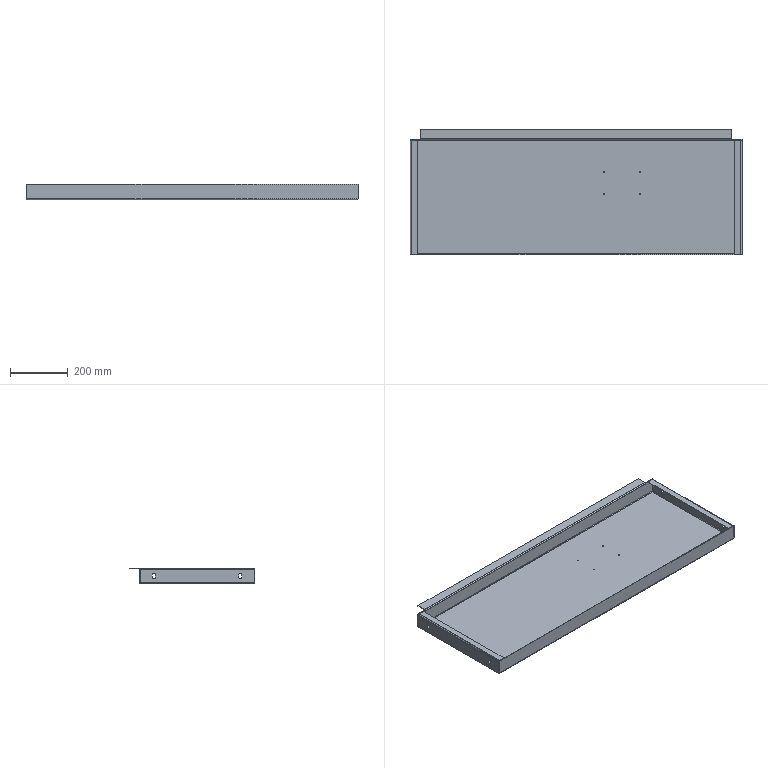Part | STEP file | SYL_0392D6J1SYL0380DJ100-914702 | 1 solid | 100 faces | box 1150 x 435 x 55 mm | volume 1345011 mm3 | plane 56 | cylinder 36 | spline 8 | commonest cylinder face diameters 10 x14 3 x8 4 x7 8 x7